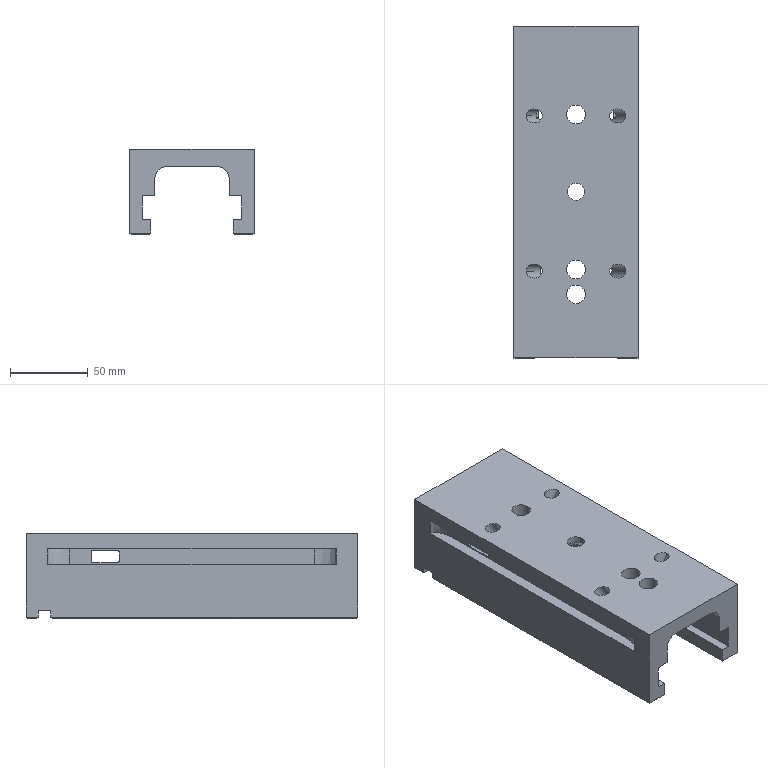Part | SolidWorks | features HoleWzd 3, ICE 3, 3DProfileFeature 2, Chamfer 1, Extrusion 1, Fillet 1, MirrorPattern 1 | 1 solid | 88 faces | box 80 x 214 x 55 mm | volume 394172 mm3 | plane 54 | cylinder 28 | spline 4 | cone 2 | commonest cylinder face diameters 2 x8 9 x8 12 x6 16 x4 11 x2